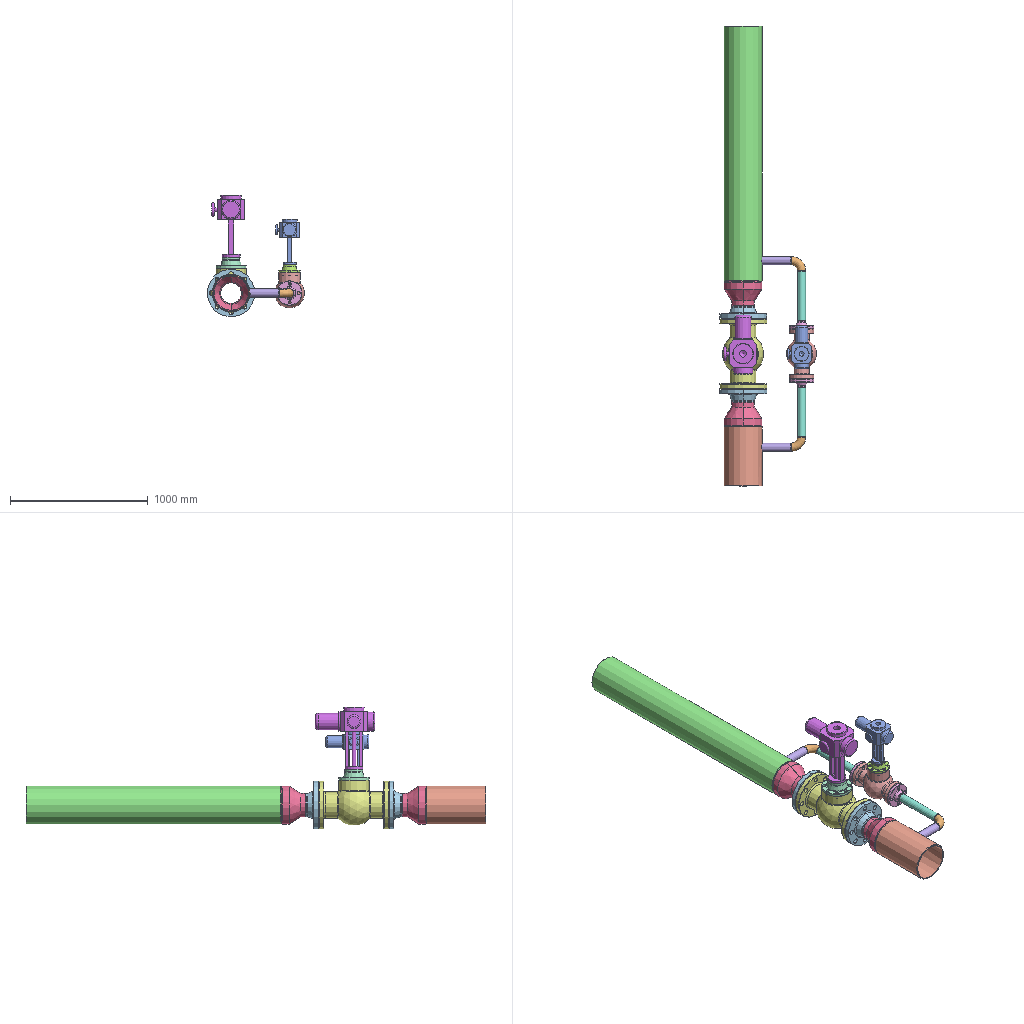Assembly | NX | 17 different items | 23 placed | box 701 x 3333 x 883 mm
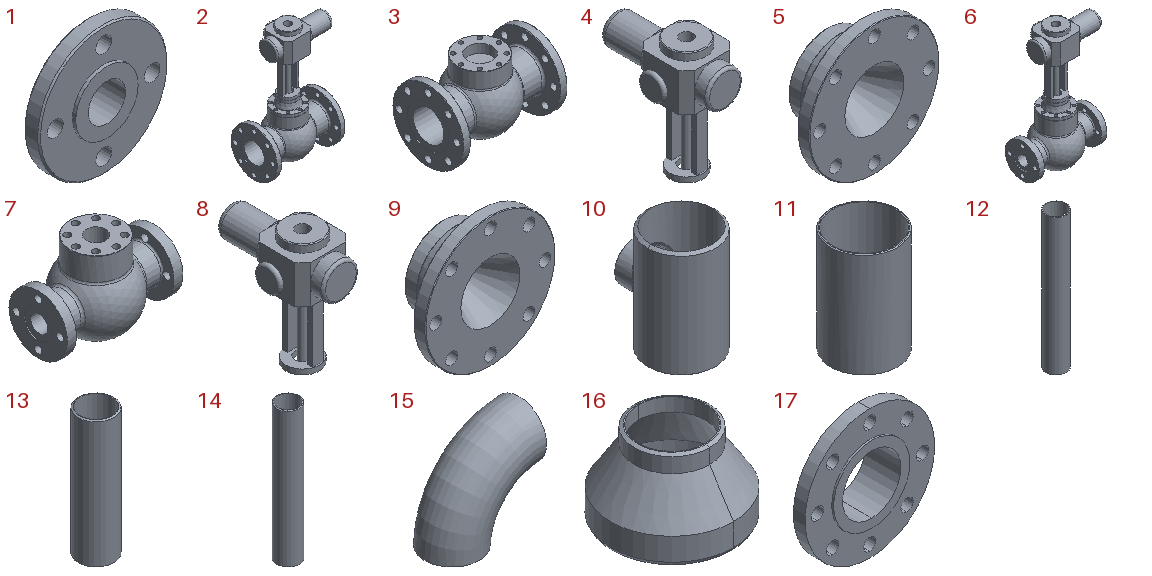Parts list (item | quantity | parent item | size | volume | features):
1 | x2 | - | 180 x 62 x 180 mm | 547253 mm3 | features DATUM_CSYS 6, SKETCH 5, EXTRACT_DATUM_AXIS 4, EXTRACT_FACE 4, HOLE PACKAGE 4, SIMPLE HOLE 4, Instance Feature 3, BLEND 1, CHAMFER 1, Pattern Feature 1, SWP104 1
2 | x1 | - | 534 x 345 x 882.5 mm | 28721924 mm3 | features INSTANCE 32, ABSOLUTE_DATUM_PLANE 11, SIMPLE HOLE 9, ABSOLUTE_DATUM_AXIS 7, CHAMFER 7, BLEND 6, BOSS 6, SKETCH 6, SWP104 6, DATUM_CSYS 5, CIRCULAR_ISET 4, HOLE PACKAGE 4, TRANSFORM_ISET 4, RECT_PAD 3, CYLINDER 2, MIRROR_SET 2, AXIS_ANGLE_DATUM_PLANE 1, EXTRUDE 1, META 1, MIRROR 1
3 | x1 | in 2 | 508 x 345 x 352.5 mm | 17565596 mm3 | features INSTANCE 24, ABSOLUTE_DATUM_AXIS 5, ABSOLUTE_DATUM_PLANE 5, SIMPLE HOLE 5, SWP104 5, CHAMFER 3, CIRCULAR_ISET 3, TRANSFORM_ISET 3, BLEND 2, MIRROR_SET 2, AXIS_ANGLE_DATUM_PLANE 1, META 1, MIRROR 1, SKETCH 1
4 | x1 | in 2 | 240 x 430 x 480 mm | 9817608 mm3 | features BOSS 6, ABSOLUTE_DATUM_PLANE 3, BLEND 3, DATUM_CSYS 3, HOLE PACKAGE 3, RECT_PAD 3, SIMPLE HOLE 3, SKETCH 3, CHAMFER 2, CYLINDER 2, ABSOLUTE_DATUM_AXIS 1, EXTRUDE 1
5 | x1 | in 2 | 220 x 80 x 220 mm | 1338664 mm3 | features INSTANCE 8, ABSOLUTE_DATUM_PLANE 3, CHAMFER 2, DATUM_CSYS 2, SKETCH 2, ABSOLUTE_DATUM_AXIS 1, BLEND 1, CIRCULAR_ISET 1, HOLE PACKAGE 1, SIMPLE HOLE 1, SWP104 1, TRANSFORM_ISET 1
6 | x1 | - | 381.638 x 220 x 645.456 mm | 12281852 mm3 | features INSTANCE 16, SIMPLE HOLE 15, SKETCH 14, DATUM_CSYS 13, HOLE PACKAGE 12, ABSOLUTE_DATUM_PLANE 11, EXTRACT_DATUM_AXIS 8, EXTRACT_FACE 8, ABSOLUTE_DATUM_AXIS 7, CHAMFER 7, BLEND 6, BOSS 6, SWP104 6, Instance Feature 3, RECT_PAD 3, Resize Face 3, CIRCULAR_ISET 2, CYLINDER 2, SCALE 2, TRANSFORM_ISET 2, AXIS_ANGLE_DATUM_PLANE 1, EXTRUDE 1, META 1, MIRROR 1, MIRROR_SET 1, Pattern Feature 1
7 | x1 | in 6 | 356 x 220 x 260 mm | 7990244 mm3 | features SIMPLE HOLE 11, SKETCH 9, DATUM_CSYS 8, EXTRACT_DATUM_AXIS 8, EXTRACT_FACE 8, HOLE PACKAGE 8, INSTANCE 8, ABSOLUTE_DATUM_AXIS 5, ABSOLUTE_DATUM_PLANE 5, SWP104 5, CHAMFER 3, Instance Feature 3, Resize Face 3, BLEND 2, AXIS_ANGLE_DATUM_PLANE 1, CIRCULAR_ISET 1, META 1, MIRROR 1, MIRROR_SET 1, Pattern Feature 1, TRANSFORM_ISET 1
8 | x1 | in 6 | 174.546 x 312.729 x 349.093 mm | 3776636 mm3 | features BOSS 6, ABSOLUTE_DATUM_PLANE 3, BLEND 3, DATUM_CSYS 3, HOLE PACKAGE 3, RECT_PAD 3, SIMPLE HOLE 3, SKETCH 3, CHAMFER 2, CYLINDER 2, ABSOLUTE_DATUM_AXIS 1, EXTRUDE 1, SCALE 1
9 | x1 | in 6 | 160 x 58.182 x 160 mm | 514948 mm3 | features INSTANCE 8, ABSOLUTE_DATUM_PLANE 3, CHAMFER 2, DATUM_CSYS 2, SKETCH 2, ABSOLUTE_DATUM_AXIS 1, BLEND 1, CIRCULAR_ISET 1, HOLE PACKAGE 1, SCALE 1, SIMPLE HOLE 1, SWP104 1, TRANSFORM_ISET 1
10 | x1 | - | 273 x 330.5 x 432 mm | 3935888 mm3 | features BREP 1
11 | x1 | - | 275 x 275 x 430 mm | 2853471 mm3 | features DATUM_CSYS 2, CHAMFER 1, CYLINDER 1, EXTRUDE 1, Resize Face 1, SHELL 1, SKETCH 1
12 | x1 | - | 275 x 275 x 1849 mm | 12376930 mm3 | features DATUM_CSYS 2, CHAMFER 1, CYLINDER 1, EXTRUDE 1, Resize Face 1, SHELL 1, SKETCH 1
13 | x2 | - | 60 x 60 x 215 mm | 114839 mm3 | features CHAMFER 2, CYLINDER 1, DATUM_CSYS 1, SHELL 1
14 | x2 | - | 60 x 60 x 361 mm | 193272 mm3 | features CHAMFER 2, CYLINDER 1, DATUM_CSYS 1, SHELL 1
15 | x2 | - | 105.988 x 60.001 x 105.988 mm | 63875 mm3 | features ABSOLUTE_DATUM_PLANE 4, ABSOLUTE_DATUM_AXIS 3, CHAMFER 2, SKETCH 1, SWP104 1
16 | x2 | - | 275 x 275 x 178 mm | 1214659 mm3 | features Resize Face 2, BREP 1
17 | x2 | - | 345 x 95 x 345 mm | 2574062 mm3 | features BREP 1, Resize Face 1
Mates (type | each side: item.copy, entity, surface, feature):
In the top assembly
Concentric | 16.1 edge | 11.1 edge
Concentric | 17.1 edge | 16.1 edge | 2 times
Concentric | 3.1 edge | 17.1 edge
Concentric | 17.1 edge | 3.1 edge
Concentric | 16.1 edge | 12.1 edge
Distance | 13.1 face plane Cylinder(1) | 12.1 face cylinder Cylinder(1)
Distance | 12.1 face cylinder Cylinder(1) | 13.1 face cylinder Cylinder(1)
Distance | 13.1 face cylinder Cylinder(1) | 12.1 face plane Cylinder(1)
Distance | 13.1 face plane Cylinder(1) | 11.1 face cylinder Cylinder(1)
Distance | 13.1 face cylinder Cylinder(1) | 11.1 face cylinder Cylinder(1)
Distance | 13.1 face cylinder Cylinder(1) | 11.1 face plane Cylinder(1)
Concentric | 15.1 edge | 13.1 edge | 2 times
Concentric | 14.1 edge | 15.1 edge | 2 times
Concentric | 14.1 edge | 1.1 edge
Concentric | 1.1 edge | 14.1 edge
Concentric | 7.1 edge | 1.1 edge
In subassembly 2
Fix | 3.1 component
Touch | 5.1 | 3.1 | 2 times
Touch | 4.1 | 5.1 | 2 times
Parallel | 4.1 | 3.1
In subassembly 6
Fix | 7.1 component
Touch | 9.1 | 7.1 | 2 times
Touch | 8.1 | 9.1 | 2 times
Parallel | 8.1 | 7.1